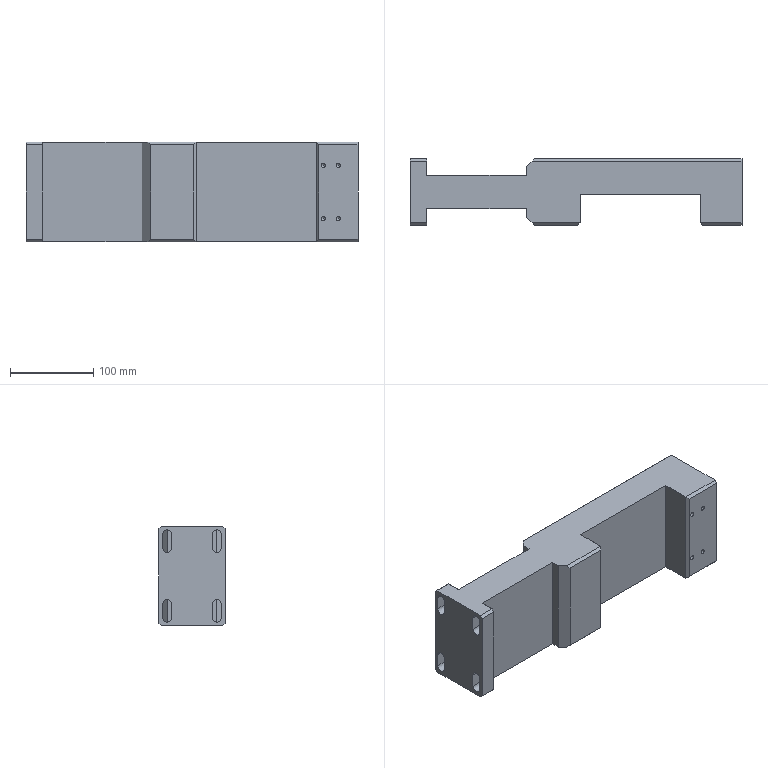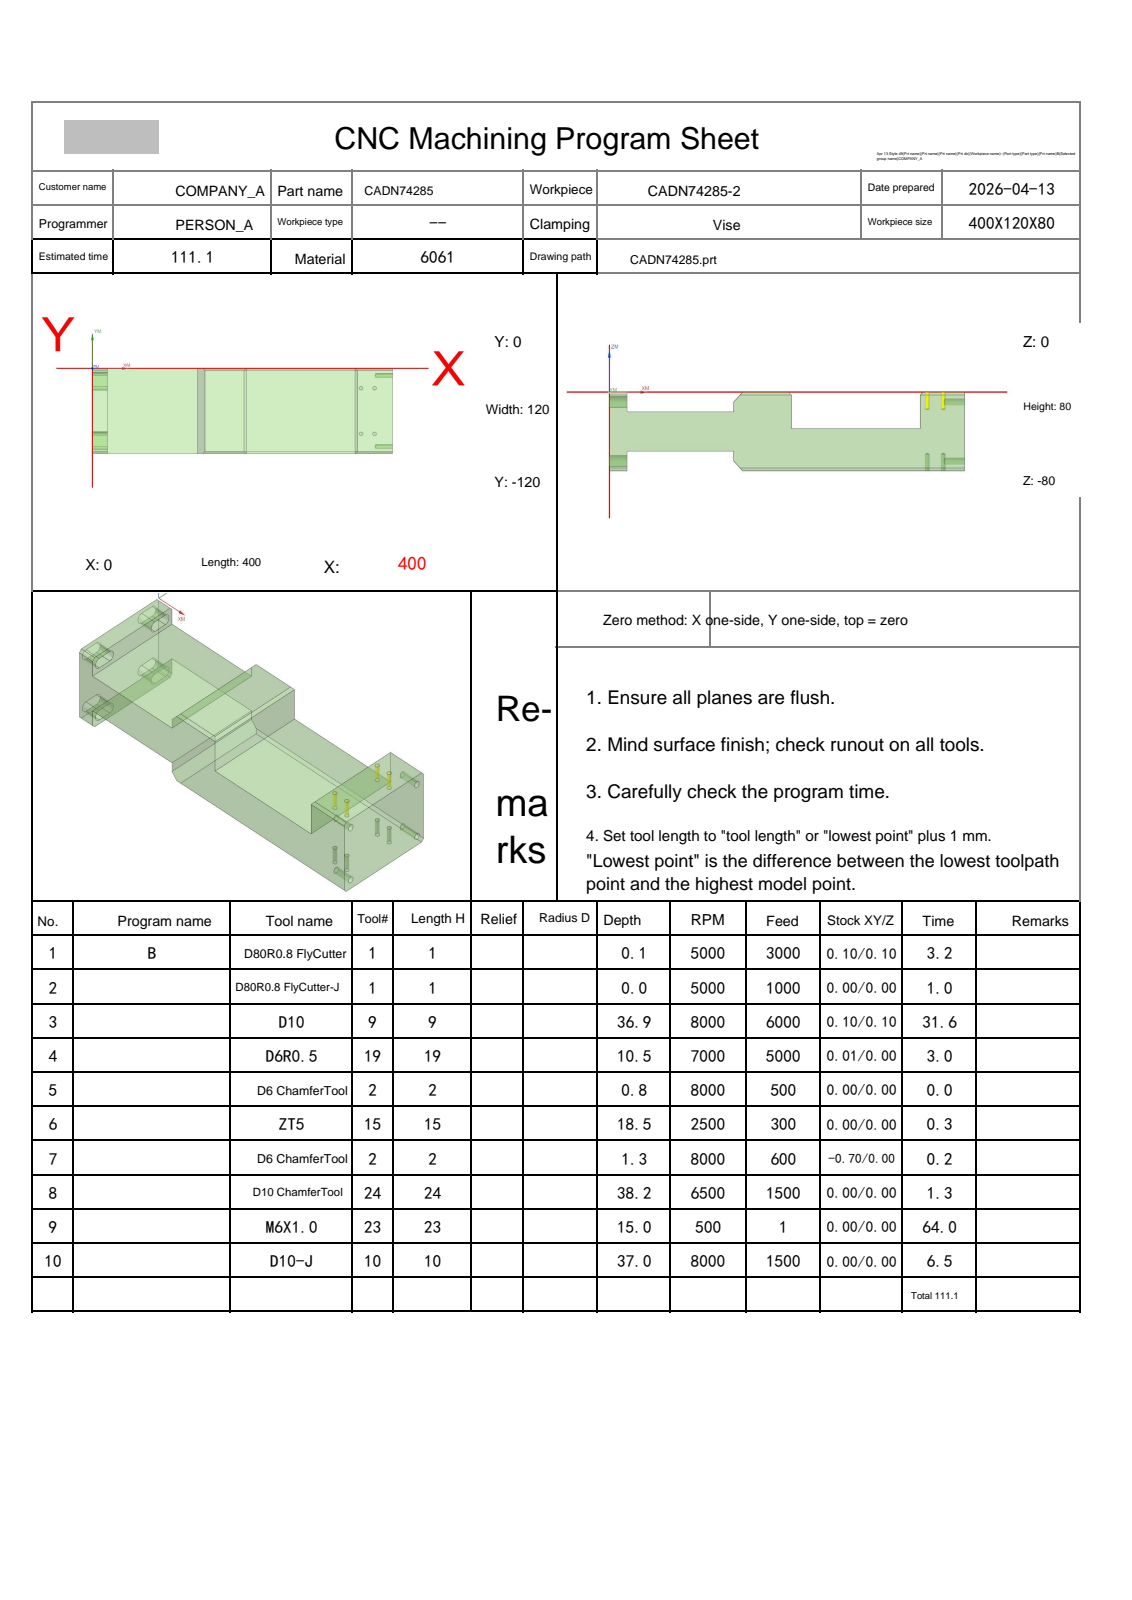NC program | NX | posted by the shop | part box 400 x 80 x 120 mm
Lines 1 to 147 of 11018:
%
O0001
(Machine time: 173.12 MIN)
(===Total Tool:8===)
(T1=D80R0.8 FlyCutter D=80.  R=0.8  D-  H01 Z=0.    )
(T9=D10     D=10.  R=0.   D-  H09 Z=-36.9 )
(T19=D6R0.5 D=6.   R=0.5  D-  H19 Z=-10.5 )
(T2=D6 ChamferTool   D=6.   R=0.   D-  H02 Z=-1.3  )
(T15=ZT5    D=5.   DR_a=118 D-  H15 Z=-18.5 )
(T24=D10 ChamferTool D=10.  R=0.   D-  H24 Z=-38.2 )
(T23=M6X1.0 D=5.   DR_a=180 D-  H23 Z=-15.  )
(T10=D10-J  D=10.  R=0.   D10 H10 Z=-37.  )
G80 G90 G17 G49 G40
G91 G28 Z0
M01
N1 T01 M06
(D80R0.8 FlyCutter  D=80. R=0.8 H=01 ce=0.10 di=0.10)
G00 G90 G54 X452.097 Y-96.097 M03 S5000
G43 H01 Z20.
M08
Z6.011
G01 Z4.011 F3000.
X440.097
X-32.101
G02 X-40.097 Y-88.101 I.004 J8.
G01 Y-39.259
G02 X-32.101 Y-31.263 I8. J-.004
G01 X440.097
X452.097
Z6.011
G00 Y-96.097
Z5.522
G01 Z3.522
X440.097
X-32.101
G02 X-40.097 Y-88.101 I.004 J8.
G01 Y-39.259
G02 X-32.101 Y-31.263 I8. J-.004
G01 X440.097
X452.097
Z5.522
G00 Y-96.097
Z5.033
G01 Z3.033
X440.097
X-32.101
G02 X-40.097 Y-88.101 I.004 J8.
G01 Y-39.259
G02 X-32.101 Y-31.263 I8. J-.004
G01 X440.097
X452.097
Z5.033
G00 Y-96.097
Z4.544
G01 Z2.544
X440.097
X-32.101
G02 X-40.097 Y-88.101 I.004 J8.
G01 Y-39.259
G02 X-32.101 Y-31.263 I8. J-.004
G01 X440.097
X452.097
Z4.544
G00 Y-96.097
Z4.056
G01 Z2.056
X440.097
X-32.101
G02 X-40.097 Y-88.101 I.004 J8.
G01 Y-39.259
G02 X-32.101 Y-31.263 I8. J-.004
G01 X440.097
X452.097
Z4.056
G00 Y-96.097
Z3.567
G01 Z1.567
X440.097
X-32.101
G02 X-40.097 Y-88.101 I.004 J8.
G01 Y-39.259
G02 X-32.101 Y-31.263 I8. J-.004
G01 X440.097
X452.097
Z3.567
G00 Y-96.097
Z3.078
G01 Z1.078
X440.097
X-32.101
G02 X-40.097 Y-88.101 I.004 J8.
G01 Y-39.259
G02 X-32.101 Y-31.263 I8. J-.004
G01 X440.097
X452.097
Z3.078
G00 Y-96.097
Z2.589
G01 Z.589
X440.097
X-32.101
G02 X-40.097 Y-88.101 I.004 J8.
G01 Y-39.259
G02 X-32.101 Y-31.263 I8. J-.004
G01 X440.097
X452.097
Z2.589
G00 Y-96.097
Z2.1
G01 Z.1
X440.097
X-32.101
G02 X-40.097 Y-88.101 I.004 J8.
G01 Y-39.259
G02 X-32.101 Y-31.263 I8. J-.004
G01 X440.097
X452.097
Z2.1
G00 Z20.
G91 G28 Z0.0
M05
M09
G91 G28 Z0.0
M01
N2 T01 M06
(D80R0.8 FlyCutter-J  D=80. R=0.8 H=01 ce=0.00 di=0.00)
G00 G90 G54 X451.999 Y-95.999 M03 S5000
G43 H01 Z20.
M08
Z2.
G01 Z0.0 F1000.
X439.999
X-32.003
G02 X-39.999 Y-88.003 I.004 J8.
G01 Y-39.357
G02 X-32.003 Y-31.361 I8. J-.004
G01 X439.999
X451.999
Z2.
G00 Z20.
G91 G28 Z0.0
M05
M09
G91 G28 Z0.0
M01